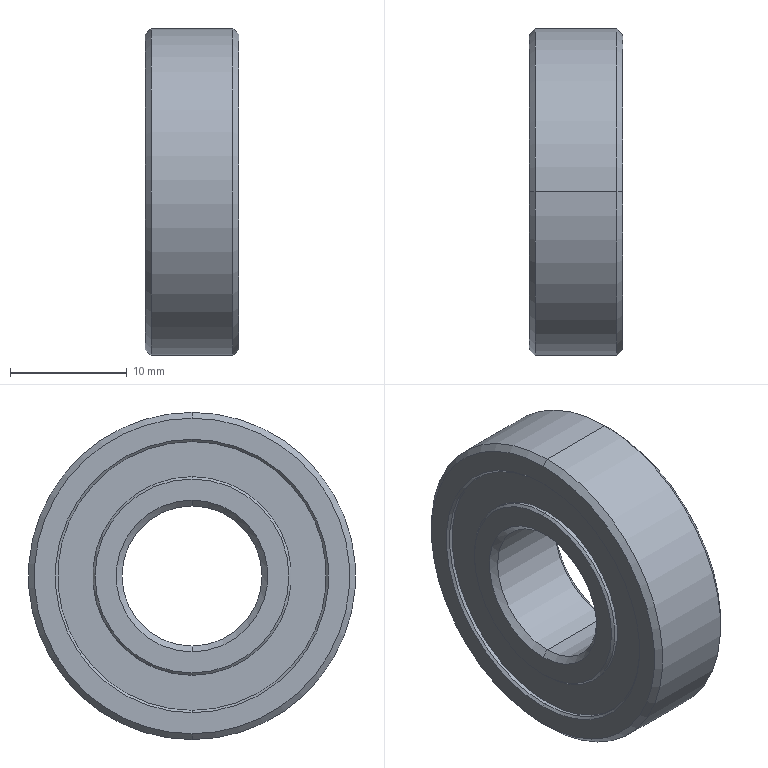Part | STEP file | 7001-1 | 1 solid | 34 faces | box 8 x 28 x 28 mm | volume 3796 mm3 | cone 16 | cylinder 12 | plane 6 | commonest cylinder face diameters 17 x4 23 x4 12 x2 28 x2